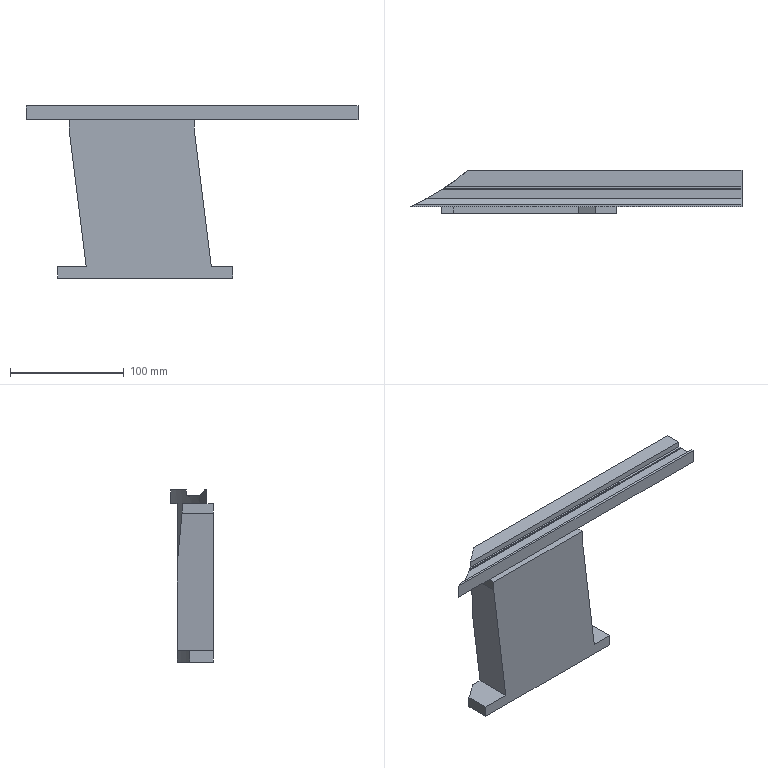Part | NX | 1 solid | 28 faces | box 291.899 x 37.727 x 151.4 mm | volume 585799 mm3 | plane 26 | cylinder 2 | commonest cylinder face diameters 412 x2
STEP:
#1=CARTESIAN_POINT('',(458.332,-185.564,-0.6));
#2=VERTEX_POINT('',#1);
#3=CARTESIAN_POINT('',(314.332,-185.564,-0.6));
#4=VERTEX_POINT('',#3);
#5=CARTESIAN_POINT('',(-273.242,-185.564,-0.6));
#6=DIRECTION('',(-1.,0.,0.));
#7=VECTOR('',#6,1000.);
#8=LINE('',#5,#7);
#9=EDGE_CURVE('',#2,#4,#8,.T.);
#10=ORIENTED_EDGE('',*,*,#9,.F.);
#11=CARTESIAN_POINT('',(458.332,-185.564,11.4));
#12=VERTEX_POINT('',#11);
#13=CARTESIAN_POINT('',(458.332,-185.564,0.));
#14=DIRECTION('',(0.,0.,1.));
#15=VECTOR('',#14,1000.);
#16=LINE('',#13,#15);
#17=EDGE_CURVE('',#2,#12,#16,.T.);
#18=ORIENTED_EDGE('',*,*,#17,.T.);
#19=CARTESIAN_POINT('',(166.433,-185.564,11.4));
#20=VERTEX_POINT('',#19);
#21=CARTESIAN_POINT('',(-273.242,-185.564,11.4));
#22=DIRECTION('',(1.,0.,0.));
#23=VECTOR('',#22,1000.);
#24=LINE('',#21,#23);
#25=EDGE_CURVE('',#20,#12,#24,.T.);
#26=ORIENTED_EDGE('',*,*,#25,.F.);
#27=CARTESIAN_POINT('',(166.433,-185.564,-0.6));
#28=VERTEX_POINT('',#27);
#29=CARTESIAN_POINT('',(166.433,-185.564,-155.14));
#30=DIRECTION('',(0.,0.,1.));
#31=VECTOR('',#30,1000.);
#32=LINE('',#29,#31);
#33=EDGE_CURVE('',#28,#20,#32,.T.);
#34=ORIENTED_EDGE('',*,*,#33,.F.);
#35=CARTESIAN_POINT('',(204.332,-185.564,-0.6));
#36=VERTEX_POINT('',#35);
#37=CARTESIAN_POINT('',(-273.242,-185.564,-0.6));
#38=DIRECTION('',(-1.,0.,0.));
#39=VECTOR('',#38,1000.);
#40=LINE('',#37,#39);
#41=EDGE_CURVE('',#36,#28,#40,.T.);
#42=ORIENTED_EDGE('',*,*,#41,.F.);
#43=CARTESIAN_POINT('',(-273.242,-185.564,-0.6));
#44=DIRECTION('',(-1.,0.,0.));
#45=VECTOR('',#44,1000.);
#46=LINE('',#43,#45);
#47=EDGE_CURVE('',#4,#36,#46,.T.);
#48=ORIENTED_EDGE('',*,*,#47,.F.);
#49=EDGE_LOOP('',(#10,#18,#26,#34,#42,#48));
#50=FACE_BOUND('',#49,.T.);
#51=CARTESIAN_POINT('',(384.332,-185.564,0.));
#52=DIRECTION('',(0.,-1.,0.));
#53=DIRECTION('',(0.,0.,-1.));
#54=AXIS2_PLACEMENT_3D('',#51,#52,#53);
#55=PLANE('',#54);
#56=ADVANCED_FACE('',(#50),#55,.T.);
#57=CARTESIAN_POINT('',(458.332,-153.564,-0.6));
#58=VERTEX_POINT('',#57);
#59=CARTESIAN_POINT('',(458.332,-346.647,-0.6));
#60=DIRECTION('',(0.,1.,0.));
#61=VECTOR('',#60,1000.);
#62=LINE('',#59,#61);
#63=EDGE_CURVE('',#2,#58,#62,.T.);
#64=ORIENTED_EDGE('',*,*,#63,.T.);
#65=CARTESIAN_POINT('',(458.332,-153.564,11.4));
#66=VERTEX_POINT('',#65);
#67=CARTESIAN_POINT('',(458.332,-153.564,0.));
#68=DIRECTION('',(0.,0.,-1.));
#69=VECTOR('',#68,1000.);
#70=LINE('',#67,#69);
#71=EDGE_CURVE('',#66,#58,#70,.T.);
#72=ORIENTED_EDGE('',*,*,#71,.F.);
#73=CARTESIAN_POINT('',(458.332,-167.364,11.4));
#74=VERTEX_POINT('',#73);
#75=CARTESIAN_POINT('',(458.332,-346.647,11.4));
#76=DIRECTION('',(0.,1.,0.));
#77=VECTOR('',#76,1000.);
#78=LINE('',#75,#77);
#79=EDGE_CURVE('',#74,#66,#78,.T.);
#80=ORIENTED_EDGE('',*,*,#79,.F.);
#81=CARTESIAN_POINT('',(458.332,-167.364,6.3));
#82=VERTEX_POINT('',#81);
#83=CARTESIAN_POINT('',(458.332,-167.364,0.));
#84=DIRECTION('',(0.,0.,-1.));
#85=VECTOR('',#84,1000.);
#86=LINE('',#83,#85);
#87=EDGE_CURVE('',#74,#82,#86,.T.);
#88=ORIENTED_EDGE('',*,*,#87,.T.);
#89=CARTESIAN_POINT('',(458.332,-169.164,6.3));
#90=VERTEX_POINT('',#89);
#91=CARTESIAN_POINT('',(458.332,-346.647,6.3));
#92=DIRECTION('',(0.,-1.,0.));
#93=VECTOR('',#92,1000.);
#94=LINE('',#91,#93);
#95=EDGE_CURVE('',#82,#90,#94,.T.);
#96=ORIENTED_EDGE('',*,*,#95,.T.);
#97=CARTESIAN_POINT('',(458.332,-169.164,5.5));
#98=VERTEX_POINT('',#97);
#99=CARTESIAN_POINT('',(458.332,-169.164,0.));
#100=DIRECTION('',(0.,0.,-1.));
#101=VECTOR('',#100,1000.);
#102=LINE('',#99,#101);
#103=EDGE_CURVE('',#90,#98,#102,.T.);
#104=ORIENTED_EDGE('',*,*,#103,.T.);
#105=CARTESIAN_POINT('',(458.332,-170.364,5.5));
#106=VERTEX_POINT('',#105);
#107=CARTESIAN_POINT('',(458.332,-346.647,5.5));
#108=DIRECTION('',(0.,-1.,0.));
#109=VECTOR('',#108,1000.);
#110=LINE('',#107,#109);
#111=EDGE_CURVE('',#98,#106,#110,.T.);
#112=ORIENTED_EDGE('',*,*,#111,.T.);
#113=CARTESIAN_POINT('',(458.332,-170.364,6.3));
#114=VERTEX_POINT('',#113);
#115=CARTESIAN_POINT('',(458.332,-170.364,0.));
#116=DIRECTION('',(0.,0.,1.));
#117=VECTOR('',#116,1000.);
#118=LINE('',#115,#117);
#119=EDGE_CURVE('',#106,#114,#118,.T.);
#120=ORIENTED_EDGE('',*,*,#119,.T.);
#121=CARTESIAN_POINT('',(458.332,-178.464,6.3));
#122=VERTEX_POINT('',#121);
#123=CARTESIAN_POINT('',(458.332,-346.647,6.3));
#124=DIRECTION('',(0.,-1.,0.));
#125=VECTOR('',#124,1000.);
#126=LINE('',#123,#125);
#127=EDGE_CURVE('',#114,#122,#126,.T.);
#128=ORIENTED_EDGE('',*,*,#127,.T.);
#129=CARTESIAN_POINT('',(458.332,-183.564,11.4));
#130=VERTEX_POINT('',#129);
#131=CARTESIAN_POINT('',(458.332,-172.164,0.));
#132=DIRECTION('',(0.,0.7071,-0.7071));
#133=VECTOR('',#132,1000.);
#134=LINE('',#131,#133);
#135=EDGE_CURVE('',#130,#122,#134,.T.);
#136=ORIENTED_EDGE('',*,*,#135,.F.);
#137=CARTESIAN_POINT('',(458.332,-346.647,11.4));
#138=DIRECTION('',(0.,1.,0.));
#139=VECTOR('',#138,1000.);
#140=LINE('',#137,#139);
#141=EDGE_CURVE('',#12,#130,#140,.T.);
#142=ORIENTED_EDGE('',*,*,#141,.F.);
#143=ORIENTED_EDGE('',*,*,#17,.F.);
#144=EDGE_LOOP('',(#64,#72,#80,#88,#96,#104,#112,#120,#128,#136,#142,#143));
#145=FACE_BOUND('',#144,.T.);
#146=CARTESIAN_POINT('',(458.332,-167.291,0.));
#147=DIRECTION('',(1.,0.,0.));
#148=DIRECTION('',(0.,1.,0.));
#149=AXIS2_PLACEMENT_3D('',#146,#147,#148);
#150=PLANE('',#149);
#151=ADVANCED_FACE('',(#145),#150,.T.);
#152=CARTESIAN_POINT('',(180.874,-178.464,6.3));
#153=VERTEX_POINT('',#152);
#154=CARTESIAN_POINT('',(194.553,-170.364,6.3));
#155=VERTEX_POINT('',#154);
#156=CARTESIAN_POINT('',(82.832,2.709,6.3));
#157=DIRECTION('',(0.,0.,1.));
#158=DIRECTION('',(1.,0.,0.));
#159=AXIS2_PLACEMENT_3D('',#156,#157,#158);
#160=CIRCLE('',#159,206.);
#161=EDGE_CURVE('',#153,#155,#160,.T.);
#162=ORIENTED_EDGE('',*,*,#161,.F.);
#163=CARTESIAN_POINT('',(-273.242,-178.464,6.3));
#164=DIRECTION('',(1.,0.,0.));
#165=VECTOR('',#164,1000.);
#166=LINE('',#163,#165);
#167=EDGE_CURVE('',#153,#122,#166,.T.);
#168=ORIENTED_EDGE('',*,*,#167,.T.);
#169=ORIENTED_EDGE('',*,*,#127,.F.);
#170=CARTESIAN_POINT('',(-273.242,-170.364,6.3));
#171=DIRECTION('',(-1.,0.,0.));
#172=VECTOR('',#171,1000.);
#173=LINE('',#170,#172);
#174=EDGE_CURVE('',#114,#155,#173,.T.);
#175=ORIENTED_EDGE('',*,*,#174,.T.);
#176=EDGE_LOOP('',(#162,#168,#169,#175));
#177=FACE_BOUND('',#176,.T.);
#178=CARTESIAN_POINT('',(99.482,-167.364,6.3));
#179=DIRECTION('',(0.,0.,-1.));
#180=DIRECTION('',(0.,-1.,0.));
#181=AXIS2_PLACEMENT_3D('',#178,#179,#180);
#182=PLANE('',#181);
#183=ADVANCED_FACE('',(#177),#182,.F.);
#184=CARTESIAN_POINT('',(204.332,-163.645,-9.));
#185=VERTEX_POINT('',#184);
#186=CARTESIAN_POINT('',(204.332,-163.645,-0.6));
#187=VERTEX_POINT('',#186);
#188=CARTESIAN_POINT('',(204.332,-163.645,-155.14));
#189=DIRECTION('',(0.,0.,1.));
#190=VECTOR('',#189,1000.);
#191=LINE('',#188,#190);
#192=EDGE_CURVE('',#185,#187,#191,.T.);
#193=ORIENTED_EDGE('',*,*,#192,.F.);
#194=CARTESIAN_POINT('',(204.332,-191.291,-9.));
#195=VERTEX_POINT('',#194);
#196=CARTESIAN_POINT('',(204.332,-175.291,-9.));
#197=DIRECTION('',(0.,-1.,0.));
#198=VECTOR('',#197,1000.);
#199=LINE('',#196,#198);
#200=EDGE_CURVE('',#185,#195,#199,.T.);
#201=ORIENTED_EDGE('',*,*,#200,.T.);
#202=CARTESIAN_POINT('',(204.332,-191.291,-0.6));
#203=VERTEX_POINT('',#202);
#204=CARTESIAN_POINT('',(204.332,-191.291,0.));
#205=DIRECTION('',(0.,0.,1.));
#206=VECTOR('',#205,1000.);
#207=LINE('',#204,#206);
#208=EDGE_CURVE('',#195,#203,#207,.T.);
#209=ORIENTED_EDGE('',*,*,#208,.T.);
#210=CARTESIAN_POINT('',(204.332,-346.647,-0.6));
#211=DIRECTION('',(0.,1.,0.));
#212=VECTOR('',#211,1000.);
#213=LINE('',#210,#212);
#214=EDGE_CURVE('',#203,#36,#213,.T.);
#215=ORIENTED_EDGE('',*,*,#214,.T.);
#216=CARTESIAN_POINT('',(204.332,-346.647,-0.6));
#217=DIRECTION('',(0.,1.,0.));
#218=VECTOR('',#217,1000.);
#219=LINE('',#216,#218);
#220=EDGE_CURVE('',#36,#187,#219,.T.);
#221=ORIENTED_EDGE('',*,*,#220,.T.);
#222=EDGE_LOOP('',(#193,#201,#209,#215,#221));
#223=FACE_BOUND('',#222,.T.);
#224=CARTESIAN_POINT('',(204.332,-175.291,-9.));
#225=DIRECTION('',(-1.,0.,0.));
#226=DIRECTION('',(0.,0.,1.));
#227=AXIS2_PLACEMENT_3D('',#224,#225,#226);
#228=PLANE('',#227);
#229=ADVANCED_FACE('',(#223),#228,.T.);
#230=CARTESIAN_POINT('',(314.332,-191.291,-0.6));
#231=VERTEX_POINT('',#230);
#232=CARTESIAN_POINT('',(314.332,-346.647,-0.6));
#233=DIRECTION('',(0.,-1.,0.));
#234=VECTOR('',#233,1000.);
#235=LINE('',#232,#234);
#236=EDGE_CURVE('',#4,#231,#235,.T.);
#237=ORIENTED_EDGE('',*,*,#236,.T.);
#238=CARTESIAN_POINT('',(314.332,-191.291,-9.));
#239=VERTEX_POINT('',#238);
#240=CARTESIAN_POINT('',(314.332,-191.291,0.));
#241=DIRECTION('',(0.,0.,-1.));
#242=VECTOR('',#241,1000.);
#243=LINE('',#240,#242);
#244=EDGE_CURVE('',#231,#239,#243,.T.);
#245=ORIENTED_EDGE('',*,*,#244,.T.);
#246=CARTESIAN_POINT('',(314.332,-159.291,-9.));
#247=VERTEX_POINT('',#246);
#248=CARTESIAN_POINT('',(314.332,-175.291,-9.));
#249=DIRECTION('',(0.,-1.,0.));
#250=VECTOR('',#249,1000.);
#251=LINE('',#248,#250);
#252=EDGE_CURVE('',#247,#239,#251,.T.);
#253=ORIENTED_EDGE('',*,*,#252,.F.);
#254=CARTESIAN_POINT('',(314.332,-159.291,-0.6));
#255=VERTEX_POINT('',#254);
#256=CARTESIAN_POINT('',(314.332,-159.291,0.));
#257=DIRECTION('',(0.,0.,-1.));
#258=VECTOR('',#257,1000.);
#259=LINE('',#256,#258);
#260=EDGE_CURVE('',#255,#247,#259,.T.);
#261=ORIENTED_EDGE('',*,*,#260,.F.);
#262=CARTESIAN_POINT('',(314.332,-346.647,-0.6));
#263=DIRECTION('',(0.,-1.,0.));
#264=VECTOR('',#263,1000.);
#265=LINE('',#262,#264);
#266=EDGE_CURVE('',#255,#4,#265,.T.);
#267=ORIENTED_EDGE('',*,*,#266,.T.);
#268=EDGE_LOOP('',(#237,#245,#253,#261,#267));
#269=FACE_BOUND('',#268,.T.);
#270=CARTESIAN_POINT('',(314.332,-175.291,0.));
#271=DIRECTION('',(1.,0.,0.));
#272=DIRECTION('',(0.,1.,0.));
#273=AXIS2_PLACEMENT_3D('',#270,#271,#272);
#274=PLANE('',#273);
#275=ADVANCED_FACE('',(#269),#274,.T.);
#276=ORIENTED_EDGE('',*,*,#244,.F.);
#277=CARTESIAN_POINT('',(-273.242,-191.291,-0.6));
#278=DIRECTION('',(-1.,0.,0.));
#279=VECTOR('',#278,1000.);
#280=LINE('',#277,#279);
#281=EDGE_CURVE('',#231,#203,#280,.T.);
#282=ORIENTED_EDGE('',*,*,#281,.T.);
#283=ORIENTED_EDGE('',*,*,#208,.F.);
#284=CARTESIAN_POINT('',(219.332,-191.291,-130.));
#285=VERTEX_POINT('',#284);
#286=CARTESIAN_POINT('',(203.216,-191.291,0.));
#287=DIRECTION('',(-0.123,0.,0.9924));
#288=VECTOR('',#287,1000.);
#289=LINE('',#286,#288);
#290=EDGE_CURVE('',#285,#195,#289,.T.);
#291=ORIENTED_EDGE('',*,*,#290,.F.);
#292=CARTESIAN_POINT('',(194.332,-191.291,-130.));
#293=VERTEX_POINT('',#292);
#294=CARTESIAN_POINT('',(-273.242,-191.291,-130.));
#295=DIRECTION('',(1.,0.,0.));
#296=VECTOR('',#295,1000.);
#297=LINE('',#294,#296);
#298=EDGE_CURVE('',#293,#285,#297,.T.);
#299=ORIENTED_EDGE('',*,*,#298,.F.);
#300=CARTESIAN_POINT('',(194.332,-191.291,-140.));
#301=VERTEX_POINT('',#300);
#302=CARTESIAN_POINT('',(194.332,-191.291,0.));
#303=DIRECTION('',(0.,0.,1.));
#304=VECTOR('',#303,1000.);
#305=LINE('',#302,#304);
#306=EDGE_CURVE('',#301,#293,#305,.T.);
#307=ORIENTED_EDGE('',*,*,#306,.F.);
#308=CARTESIAN_POINT('',(348.332,-191.291,-140.));
#309=VERTEX_POINT('',#308);
#310=CARTESIAN_POINT('',(-273.242,-191.291,-140.));
#311=DIRECTION('',(-1.,0.,0.));
#312=VECTOR('',#311,1000.);
#313=LINE('',#310,#312);
#314=EDGE_CURVE('',#309,#301,#313,.T.);
#315=ORIENTED_EDGE('',*,*,#314,.F.);
#316=CARTESIAN_POINT('',(348.332,-191.291,-130.));
#317=VERTEX_POINT('',#316);
#318=CARTESIAN_POINT('',(348.332,-191.291,0.));
#319=DIRECTION('',(0.,0.,-1.));
#320=VECTOR('',#319,1000.);
#321=LINE('',#318,#320);
#322=EDGE_CURVE('',#317,#309,#321,.T.);
#323=ORIENTED_EDGE('',*,*,#322,.F.);
#324=CARTESIAN_POINT('',(329.332,-191.291,-130.));
#325=VERTEX_POINT('',#324);
#326=CARTESIAN_POINT('',(-273.242,-191.291,-130.));
#327=DIRECTION('',(1.,0.,0.));
#328=VECTOR('',#327,1000.);
#329=LINE('',#326,#328);
#330=EDGE_CURVE('',#325,#317,#329,.T.);
#331=ORIENTED_EDGE('',*,*,#330,.F.);
#332=CARTESIAN_POINT('',(313.216,-191.291,0.));
#333=DIRECTION('',(0.123,0.,-0.9924));
#334=VECTOR('',#333,1000.);
#335=LINE('',#332,#334);
#336=EDGE_CURVE('',#239,#325,#335,.T.);
#337=ORIENTED_EDGE('',*,*,#336,.F.);
#338=EDGE_LOOP('',(#276,#282,#283,#291,#299,#307,#315,#323,#331,#337));
#339=FACE_BOUND('',#338,.T.);
#340=CARTESIAN_POINT('',(377.274,-191.291,2.035));
#341=DIRECTION('',(0.,-1.,0.));
#342=DIRECTION('',(0.,0.,-1.));
#343=AXIS2_PLACEMENT_3D('',#340,#341,#342);
#344=PLANE('',#343);
#345=ADVANCED_FACE('',(#339),#344,.T.);
#346=CARTESIAN_POINT('',(348.332,-159.291,-140.));
#347=VERTEX_POINT('',#346);
#348=CARTESIAN_POINT('',(348.332,-346.647,-140.));
#349=DIRECTION('',(0.,-1.,0.));
#350=VECTOR('',#349,1000.);
#351=LINE('',#348,#350);
#352=EDGE_CURVE('',#347,#309,#351,.T.);
#353=ORIENTED_EDGE('',*,*,#352,.F.);
#354=CARTESIAN_POINT('',(348.332,-159.291,-130.));
#355=VERTEX_POINT('',#354);
#356=CARTESIAN_POINT('',(348.332,-159.291,0.));
#357=DIRECTION('',(0.,0.,-1.));
#358=VECTOR('',#357,1000.);
#359=LINE('',#356,#358);
#360=EDGE_CURVE('',#355,#347,#359,.T.);
#361=ORIENTED_EDGE('',*,*,#360,.F.);
#362=CARTESIAN_POINT('',(348.332,-346.647,-130.));
#363=DIRECTION('',(0.,-1.,0.));
#364=VECTOR('',#363,1000.);
#365=LINE('',#362,#364);
#366=EDGE_CURVE('',#355,#317,#365,.T.);
#367=ORIENTED_EDGE('',*,*,#366,.T.);
#368=ORIENTED_EDGE('',*,*,#322,.T.);
#369=EDGE_LOOP('',(#353,#361,#367,#368));
#370=FACE_BOUND('',#369,.T.);
#371=CARTESIAN_POINT('',(348.332,-175.291,-140.));
#372=DIRECTION('',(1.,0.,0.));
#373=DIRECTION('',(0.,1.,0.));
#374=AXIS2_PLACEMENT_3D('',#371,#372,#373);
#375=PLANE('',#374);
#376=ADVANCED_FACE('',(#370),#375,.T.);
#377=CARTESIAN_POINT('',(194.332,-170.507,-130.));
#378=VERTEX_POINT('',#377);
#379=CARTESIAN_POINT('',(210.08,-159.291,-130.));
#380=VERTEX_POINT('',#379);
#381=CARTESIAN_POINT('',(82.832,2.709,-130.));
#382=DIRECTION('',(0.,0.,1.));
#383=DIRECTION('',(1.,0.,0.));
#384=AXIS2_PLACEMENT_3D('',#381,#382,#383);
#385=CIRCLE('',#384,206.);
#386=EDGE_CURVE('',#378,#380,#385,.T.);
#387=ORIENTED_EDGE('',*,*,#386,.F.);
#388=CARTESIAN_POINT('',(194.332,-175.291,-130.));
#389=DIRECTION('',(0.,1.,0.));
#390=VECTOR('',#389,1000.);
#391=LINE('',#388,#390);
#392=EDGE_CURVE('',#293,#378,#391,.T.);
#393=ORIENTED_EDGE('',*,*,#392,.F.);
#394=ORIENTED_EDGE('',*,*,#298,.T.);
#395=CARTESIAN_POINT('',(219.332,-159.291,-130.));
#396=VERTEX_POINT('',#395);
#397=CARTESIAN_POINT('',(219.332,-346.647,-130.));
#398=DIRECTION('',(0.,1.,0.));
#399=VECTOR('',#398,1000.);
#400=LINE('',#397,#399);
#401=EDGE_CURVE('',#285,#396,#400,.T.);
#402=ORIENTED_EDGE('',*,*,#401,.T.);
#403=CARTESIAN_POINT('',(-273.242,-159.291,-130.));
#404=DIRECTION('',(1.,0.,0.));
#405=VECTOR('',#404,1000.);
#406=LINE('',#403,#405);
#407=EDGE_CURVE('',#380,#396,#406,.T.);
#408=ORIENTED_EDGE('',*,*,#407,.F.);
#409=EDGE_LOOP('',(#387,#393,#394,#402,#408));
#410=FACE_BOUND('',#409,.T.);
#411=CARTESIAN_POINT('',(194.332,-175.291,-130.));
#412=DIRECTION('',(0.,0.,1.));
#413=DIRECTION('',(1.,0.,0.));
#414=AXIS2_PLACEMENT_3D('',#411,#412,#413);
#415=PLANE('',#414);
#416=ADVANCED_FACE('',(#410),#415,.T.);
#417=CARTESIAN_POINT('',(329.332,-159.291,-130.));
#418=VERTEX_POINT('',#417);
#419=CARTESIAN_POINT('',(329.332,-346.647,-130.));
#420=DIRECTION('',(0.,-1.,0.));
#421=VECTOR('',#420,1000.);
#422=LINE('',#419,#421);
#423=EDGE_CURVE('',#418,#325,#422,.T.);
#424=ORIENTED_EDGE('',*,*,#423,.F.);
#425=CARTESIAN_POINT('',(313.216,-159.291,0.));
#426=DIRECTION('',(0.123,0.,-0.9924));
#427=VECTOR('',#426,1000.);
#428=LINE('',#425,#427);
#429=EDGE_CURVE('',#247,#418,#428,.T.);
#430=ORIENTED_EDGE('',*,*,#429,.F.);
#431=ORIENTED_EDGE('',*,*,#252,.T.);
#432=ORIENTED_EDGE('',*,*,#336,.T.);
#433=EDGE_LOOP('',(#424,#430,#431,#432));
#434=FACE_BOUND('',#433,.T.);
#435=CARTESIAN_POINT('',(329.332,-175.291,-130.));
#436=DIRECTION('',(0.9924,0.,0.123));
#437=DIRECTION('',(0.,-1.,0.));
#438=AXIS2_PLACEMENT_3D('',#435,#436,#437);
#439=PLANE('',#438);
#440=ADVANCED_FACE('',(#434),#439,.T.);
#441=ORIENTED_EDGE('',*,*,#47,.T.);
#442=ORIENTED_EDGE('',*,*,#214,.F.);
#443=ORIENTED_EDGE('',*,*,#281,.F.);
#444=ORIENTED_EDGE('',*,*,#236,.F.);
#445=EDGE_LOOP('',(#441,#442,#443,#444));
#446=FACE_BOUND('',#445,.T.);
#447=CARTESIAN_POINT('',(204.332,-175.291,-0.6));
#448=DIRECTION('',(0.,0.,1.));
#449=DIRECTION('',(1.,0.,0.));
#450=AXIS2_PLACEMENT_3D('',#447,#448,#449);
#451=PLANE('',#450);
#452=ADVANCED_FACE('',(#446),#451,.T.);
#453=CARTESIAN_POINT('',(210.08,-159.291,-55.366));
#454=VERTEX_POINT('',#453);
#455=CARTESIAN_POINT('',(210.08,-159.291,-0.6));
#456=VERTEX_POINT('',#455);
#457=CARTESIAN_POINT('',(210.08,-159.291,-155.14));
#458=DIRECTION('',(0.,0.,1.));
#459=VECTOR('',#458,1000.);
#460=LINE('',#457,#459);
#461=EDGE_CURVE('',#454,#456,#460,.T.);
#462=ORIENTED_EDGE('',*,*,#461,.T.);
#463=CARTESIAN_POINT('',(-273.242,-159.291,-0.6));
#464=DIRECTION('',(-1.,0.,0.));
#465=VECTOR('',#464,1000.);
#466=LINE('',#463,#465);
#467=EDGE_CURVE('',#255,#456,#466,.T.);
#468=ORIENTED_EDGE('',*,*,#467,.F.);
#469=ORIENTED_EDGE('',*,*,#260,.T.);
#470=ORIENTED_EDGE('',*,*,#429,.T.);
#471=CARTESIAN_POINT('',(-273.242,-159.291,-130.));
#472=DIRECTION('',(-1.,0.,0.));
#473=VECTOR('',#472,1000.);
#474=LINE('',#471,#473);
#475=EDGE_CURVE('',#355,#418,#474,.T.);
#476=ORIENTED_EDGE('',*,*,#475,.F.);
#477=ORIENTED_EDGE('',*,*,#360,.T.);
#478=CARTESIAN_POINT('',(210.08,-159.291,-140.));
#479=VERTEX_POINT('',#478);
#480=CARTESIAN_POINT('',(-273.242,-159.291,-140.));
#481=DIRECTION('',(-1.,0.,0.));
#482=VECTOR('',#481,1000.);
#483=LINE('',#480,#482);
#484=EDGE_CURVE('',#347,#479,#483,.T.);
#485=ORIENTED_EDGE('',*,*,#484,.T.);
#486=CARTESIAN_POINT('',(210.08,-159.291,-155.14));
#487=DIRECTION('',(0.,0.,1.));
#488=VECTOR('',#487,1000.);
#489=LINE('',#486,#488);
#490=EDGE_CURVE('',#479,#380,#489,.T.);
#491=ORIENTED_EDGE('',*,*,#490,.T.);
#492=ORIENTED_EDGE('',*,*,#407,.T.);
#493=CARTESIAN_POINT('',(203.216,-159.291,0.));
#494=DIRECTION('',(-0.123,0.,0.9924));
#495=VECTOR('',#494,1000.);
#496=LINE('',#493,#495);
#497=EDGE_CURVE('',#396,#454,#496,.T.);
#498=ORIENTED_EDGE('',*,*,#497,.T.);
#499=EDGE_LOOP('',(#462,#468,#469,#470,#476,#477,#485,#491,#492,#498));
#500=FACE_BOUND('',#499,.T.);
#501=CARTESIAN_POINT('',(377.274,-159.291,2.035));
#502=DIRECTION('',(0.,-1.,0.));
#503=DIRECTION('',(0.,0.,-1.));
#504=AXIS2_PLACEMENT_3D('',#501,#502,#503);
#505=PLANE('',#504);
#506=ADVANCED_FACE('',(#500),#505,.F.);
#507=CARTESIAN_POINT('',(217.05,-153.564,-0.6));
#508=VERTEX_POINT('',#507);
#509=CARTESIAN_POINT('',(217.05,-153.564,11.4));
#510=VERTEX_POINT('',#509);
#511=CARTESIAN_POINT('',(217.05,-153.564,-155.14));
#512=DIRECTION('',(0.,0.,1.));
#513=VECTOR('',#512,1000.);
#514=LINE('',#511,#513);
#515=EDGE_CURVE('',#508,#510,#514,.T.);
#516=ORIENTED_EDGE('',*,*,#515,.T.);
#517=CARTESIAN_POINT('',(-273.242,-153.564,11.4));
#518=DIRECTION('',(-1.,0.,0.));
#519=VECTOR('',#518,1000.);
#520=LINE('',#517,#519);
#521=EDGE_CURVE('',#66,#510,#520,.T.);
#522=ORIENTED_EDGE('',*,*,#521,.F.);
#523=ORIENTED_EDGE('',*,*,#71,.T.);
#524=CARTESIAN_POINT('',(-273.242,-153.564,-0.6));
#525=DIRECTION('',(1.,0.,0.));
#526=VECTOR('',#525,1000.);
#527=LINE('',#524,#526);
#528=EDGE_CURVE('',#508,#58,#527,.T.);
#529=ORIENTED_EDGE('',*,*,#528,.F.);
#530=EDGE_LOOP('',(#516,#522,#523,#529));
#531=FACE_BOUND('',#530,.T.);
#532=CARTESIAN_POINT('',(134.332,-153.564,0.));
#533=DIRECTION('',(0.,1.,0.));
#534=DIRECTION('',(1.,0.,0.));
#535=AXIS2_PLACEMENT_3D('',#532,#533,#534);
#536=PLANE('',#535);
#537=ADVANCED_FACE('',(#531),#536,.T.);
#538=ORIENTED_EDGE('',*,*,#200,.F.);
#539=CARTESIAN_POINT('',(210.08,-159.291,-55.366));
#540=CARTESIAN_POINT('',(208.189,-160.776,-40.116));
#541=CARTESIAN_POINT('',(206.273,-162.227,-24.659));
#542=CARTESIAN_POINT('',(204.332,-163.645,-9.));
#543=(BOUNDED_CURVE()B_SPLINE_CURVE(3,(#539,#540,#541,#542),.UNSPECIFIED.,.F.,.F.)B_SPLINE_CURVE_WITH_KNOTS((4,4),(4.047,4.082),.UNSPECIFIED.)CURVE()GEOMETRIC_REPRESENTATION_ITEM()RATIONAL_B_SPLINE_CURVE((1.,0.9999,0.9999,1.))REPRESENTATION_ITEM(''));
#544=EDGE_CURVE('',#454,#185,#543,.T.);
#545=ORIENTED_EDGE('',*,*,#544,.F.);
#546=ORIENTED_EDGE('',*,*,#497,.F.);
#547=ORIENTED_EDGE('',*,*,#401,.F.);
#548=ORIENTED_EDGE('',*,*,#290,.T.);
#549=EDGE_LOOP('',(#538,#545,#546,#547,#548));
#550=FACE_BOUND('',#549,.T.);
#551=CARTESIAN_POINT('',(204.332,-175.291,-9.));
#552=DIRECTION('',(-0.9924,0.,-0.123));
#553=DIRECTION('',(-0.123,0.,0.9924));
#554=AXIS2_PLACEMENT_3D('',#551,#552,#553);
#555=PLANE('',#554);
#556=ADVANCED_FACE('',(#550),#555,.T.);
#557=CARTESIAN_POINT('',(194.332,-170.507,-140.));
#558=VERTEX_POINT('',#557);
#559=CARTESIAN_POINT('',(194.332,-346.647,-140.));
#560=DIRECTION('',(0.,-1.,0.));
#561=VECTOR('',#560,1000.);
#562=LINE('',#559,#561);
#563=EDGE_CURVE('',#558,#301,#562,.T.);
#564=ORIENTED_EDGE('',*,*,#563,.T.);
#565=ORIENTED_EDGE('',*,*,#306,.T.);
#566=ORIENTED_EDGE('',*,*,#392,.T.);
#567=CARTESIAN_POINT('',(194.332,-170.507,-155.14));
#568=DIRECTION('',(0.,0.,1.));
#569=VECTOR('',#568,1000.);
#570=LINE('',#567,#569);
#571=EDGE_CURVE('',#558,#378,#570,.T.);
#572=ORIENTED_EDGE('',*,*,#571,.F.);
#573=EDGE_LOOP('',(#564,#565,#566,#572));
#574=FACE_BOUND('',#573,.T.);
#575=CARTESIAN_POINT('',(194.332,-175.291,-140.));
#576=DIRECTION('',(-1.,0.,0.));
#577=DIRECTION('',(0.,0.,1.));
#578=AXIS2_PLACEMENT_3D('',#575,#576,#577);
#579=PLANE('',#578);
#580=ADVANCED_FACE('',(#574),#579,.T.);
#581=ORIENTED_EDGE('',*,*,#563,.F.);
#582=CARTESIAN_POINT('',(82.832,2.709,-140.));
#583=DIRECTION('',(0.,0.,1.));
#584=DIRECTION('',(1.,0.,0.));
#585=AXIS2_PLACEMENT_3D('',#582,#583,#584);
#586=CIRCLE('',#585,206.);
#587=EDGE_CURVE('',#558,#479,#586,.T.);
#588=ORIENTED_EDGE('',*,*,#587,.T.);
#589=ORIENTED_EDGE('',*,*,#484,.F.);
#590=ORIENTED_EDGE('',*,*,#352,.T.);
#591=ORIENTED_EDGE('',*,*,#314,.T.);
#592=EDGE_LOOP('',(#581,#588,#589,#590,#591));
#593=FACE_BOUND('',#592,.T.);
#594=CARTESIAN_POINT('',(194.332,-175.291,-140.));
#595=DIRECTION('',(0.,0.,-1.));
#596=DIRECTION('',(0.,-1.,0.));
#597=AXIS2_PLACEMENT_3D('',#594,#595,#596);
#598=PLANE('',#597);
#599=ADVANCED_FACE('',(#593),#598,.T.);
#600=ORIENTED_EDGE('',*,*,#423,.T.);
#601=ORIENTED_EDGE('',*,*,#330,.T.);
#602=ORIENTED_EDGE('',*,*,#366,.F.);
#603=ORIENTED_EDGE('',*,*,#475,.T.);
#604=EDGE_LOOP('',(#600,#601,#602,#603));
#605=FACE_BOUND('',#604,.T.);
#606=CARTESIAN_POINT('',(354.332,-175.291,-130.));
#607=DIRECTION('',(0.,0.,1.));
#608=DIRECTION('',(1.,0.,0.));
#609=AXIS2_PLACEMENT_3D('',#606,#607,#608);
#610=PLANE('',#609);
#611=ADVANCED_FACE('',(#605),#610,.T.);
#612=ORIENTED_EDGE('',*,*,#167,.F.);
#613=CARTESIAN_POINT('',(170.799,-183.564,11.4));
#614=VERTEX_POINT('',#613);
#615=CARTESIAN_POINT('',(170.799,-183.564,11.4));
#616=CARTESIAN_POINT('',(174.203,-181.957,9.792));
#617=CARTESIAN_POINT('',(177.562,-180.256,8.092));
#618=CARTESIAN_POINT('',(180.874,-178.464,6.3));
#619=(BOUNDED_CURVE()B_SPLINE_CURVE(3,(#615,#616,#617,#618),.UNSPECIFIED.,.F.,.F.)B_SPLINE_CURVE_WITH_KNOTS((4,4),(0.4412,0.496),.UNSPECIFIED.)CURVE()GEOMETRIC_REPRESENTATION_ITEM()RATIONAL_B_SPLINE_CURVE((1.,0.9997,0.9997,1.))REPRESENTATION_ITEM(''));
#620=EDGE_CURVE('',#614,#153,#619,.T.);
#621=ORIENTED_EDGE('',*,*,#620,.F.);
#622=CARTESIAN_POINT('',(-273.242,-183.564,11.4));
#623=DIRECTION('',(1.,0.,0.));
#624=VECTOR('',#623,1000.);
#625=LINE('',#622,#624);
#626=EDGE_CURVE('',#614,#130,#625,.T.);
#627=ORIENTED_EDGE('',*,*,#626,.T.);
#628=ORIENTED_EDGE('',*,*,#135,.T.);
#629=EDGE_LOOP('',(#612,#621,#627,#628));
#630=FACE_BOUND('',#629,.T.);
#631=CARTESIAN_POINT('',(308.582,-181.014,8.85));
#632=DIRECTION('',(0.,0.7071,0.7071));
#633=DIRECTION('',(1.,0.,0.));
#634=AXIS2_PLACEMENT_3D('',#631,#632,#633);
#635=PLANE('',#634);
#636=ADVANCED_FACE('',(#630),#635,.T.);
#637=ORIENTED_EDGE('',*,*,#87,.F.);
#638=CARTESIAN_POINT('',(199.069,-167.364,11.4));
#639=VERTEX_POINT('',#638);
#640=CARTESIAN_POINT('',(-273.242,-167.364,11.4));
#641=DIRECTION('',(-1.,0.,0.));
#642=VECTOR('',#641,1000.);
#643=LINE('',#640,#642);
#644=EDGE_CURVE('',#74,#639,#643,.T.);
#645=ORIENTED_EDGE('',*,*,#644,.T.);
#646=CARTESIAN_POINT('',(199.069,-167.364,6.3));
#647=VERTEX_POINT('',#646);
#648=CARTESIAN_POINT('',(199.069,-167.364,-155.14));
#649=DIRECTION('',(0.,0.,1.));
#650=VECTOR('',#649,1000.);
#651=LINE('',#648,#650);
#652=EDGE_CURVE('',#647,#639,#651,.T.);
#653=ORIENTED_EDGE('',*,*,#652,.F.);
#654=CARTESIAN_POINT('',(-273.242,-167.364,6.3));
#655=DIRECTION('',(1.,0.,0.));
#656=VECTOR('',#655,1000.);
#657=LINE('',#654,#656);
#658=EDGE_CURVE('',#647,#82,#657,.T.);
#659=ORIENTED_EDGE('',*,*,#658,.T.);
#660=EDGE_LOOP('',(#637,#645,#653,#659));
#661=FACE_BOUND('',#660,.T.);
#662=CARTESIAN_POINT('',(99.482,-167.364,20.8));
#663=DIRECTION('',(0.,1.,0.));
#664=DIRECTION('',(1.,0.,0.));
#665=AXIS2_PLACEMENT_3D('',#662,#663,#664);
#666=PLANE('',#665);
#667=ADVANCED_FACE('',(#661),#666,.F.);
#668=CARTESIAN_POINT('',(194.553,-170.364,5.5));
#669=VERTEX_POINT('',#668);
#670=CARTESIAN_POINT('',(196.39,-169.164,5.5));
#671=VERTEX_POINT('',#670);
#672=CARTESIAN_POINT('',(82.832,2.709,5.5));
#673=DIRECTION('',(0.,0.,1.));
#674=DIRECTION('',(1.,0.,0.));
#675=AXIS2_PLACEMENT_3D('',#672,#673,#674);
#676=CIRCLE('',#675,206.);
#677=EDGE_CURVE('',#669,#671,#676,.T.);
#678=ORIENTED_EDGE('',*,*,#677,.F.);
#679=CARTESIAN_POINT('',(-273.242,-170.364,5.5));
#680=DIRECTION('',(1.,0.,0.));
#681=VECTOR('',#680,1000.);
#682=LINE('',#679,#681);
#683=EDGE_CURVE('',#669,#106,#682,.T.);
#684=ORIENTED_EDGE('',*,*,#683,.T.);
#685=ORIENTED_EDGE('',*,*,#111,.F.);
#686=CARTESIAN_POINT('',(-273.242,-169.164,5.5));
#687=DIRECTION('',(1.,0.,0.));
#688=VECTOR('',#687,1000.);
#689=LINE('',#686,#688);
#690=EDGE_CURVE('',#671,#98,#689,.T.);
#691=ORIENTED_EDGE('',*,*,#690,.F.);
#692=EDGE_LOOP('',(#678,#684,#685,#691));
#693=FACE_BOUND('',#692,.T.);
#694=CARTESIAN_POINT('',(99.482,-169.164,5.5));
#695=DIRECTION('',(0.,0.,-1.));
#696=DIRECTION('',(0.,-1.,0.));
#697=AXIS2_PLACEMENT_3D('',#694,#695,#696);
#698=PLANE('',#697);
#699=ADVANCED_FACE('',(#693),#698,.F.);
#700=CARTESIAN_POINT('',(196.39,-169.164,6.3));
#701=VERTEX_POINT('',#700);
#702=CARTESIAN_POINT('',(-273.242,-169.164,6.3));
#703=DIRECTION('',(1.,0.,0.));
#704=VECTOR('',#703,1000.);
#705=LINE('',#702,#704);
#706=EDGE_CURVE('',#701,#90,#705,.T.);
#707=ORIENTED_EDGE('',*,*,#706,.T.);
#708=ORIENTED_EDGE('',*,*,#95,.F.);
#709=ORIENTED_EDGE('',*,*,#658,.F.);
#710=CARTESIAN_POINT('',(82.832,2.709,6.3));
#711=DIRECTION('',(0.,0.,1.));
#712=DIRECTION('',(1.,0.,0.));
#713=AXIS2_PLACEMENT_3D('',#710,#711,#712);
#714=CIRCLE('',#713,206.);
#715=EDGE_CURVE('',#701,#647,#714,.T.);
#716=ORIENTED_EDGE('',*,*,#715,.F.);
#717=EDGE_LOOP('',(#707,#708,#709,#716));
#718=FACE_BOUND('',#717,.T.);
#719=CARTESIAN_POINT('',(99.482,-167.364,6.3));
#720=DIRECTION('',(0.,0.,-1.));
#721=DIRECTION('',(0.,-1.,0.));
#722=AXIS2_PLACEMENT_3D('',#719,#720,#721);
#723=PLANE('',#722);
#724=ADVANCED_FACE('',(#718),#723,.F.);
#725=ORIENTED_EDGE('',*,*,#119,.F.);
#726=ORIENTED_EDGE('',*,*,#683,.F.);
#727=CARTESIAN_POINT('',(194.553,-170.364,-155.14));
#728=DIRECTION('',(0.,0.,1.));
#729=VECTOR('',#728,1000.);
#730=LINE('',#727,#729);
#731=EDGE_CURVE('',#669,#155,#730,.T.);
#732=ORIENTED_EDGE('',*,*,#731,.T.);
#733=ORIENTED_EDGE('',*,*,#174,.F.);
#734=EDGE_LOOP('',(#725,#726,#732,#733));
#735=FACE_BOUND('',#734,.T.);
#736=CARTESIAN_POINT('',(99.482,-170.364,5.5));
#737=DIRECTION('',(0.,-1.,0.));
#738=DIRECTION('',(0.,0.,-1.));
#739=AXIS2_PLACEMENT_3D('',#736,#737,#738);
#740=PLANE('',#739);
#741=ADVANCED_FACE('',(#735),#740,.F.);
#742=ORIENTED_EDGE('',*,*,#103,.F.);
#743=ORIENTED_EDGE('',*,*,#706,.F.);
#744=CARTESIAN_POINT('',(196.39,-169.164,-155.14));
#745=DIRECTION('',(0.,0.,1.));
#746=VECTOR('',#745,1000.);
#747=LINE('',#744,#746);
#748=EDGE_CURVE('',#671,#701,#747,.T.);
#749=ORIENTED_EDGE('',*,*,#748,.F.);
#750=ORIENTED_EDGE('',*,*,#690,.T.);
#751=EDGE_LOOP('',(#742,#743,#749,#750));
#752=FACE_BOUND('',#751,.T.);
#753=CARTESIAN_POINT('',(99.482,-169.164,6.3));
#754=DIRECTION('',(0.,1.,0.));
#755=DIRECTION('',(1.,0.,0.));
#756=AXIS2_PLACEMENT_3D('',#753,#754,#755);
#757=PLANE('',#756);
#758=ADVANCED_FACE('',(#752),#757,.F.);
#759=ORIENTED_EDGE('',*,*,#571,.T.);
#760=ORIENTED_EDGE('',*,*,#386,.T.);
#761=ORIENTED_EDGE('',*,*,#490,.F.);
#762=ORIENTED_EDGE('',*,*,#587,.F.);
#763=EDGE_LOOP('',(#759,#760,#761,#762));
#764=FACE_BOUND('',#763,.T.);
#765=CARTESIAN_POINT('',(82.832,2.709,-155.14));
#766=DIRECTION('',(0.,0.,1.));
#767=DIRECTION('',(1.,0.,0.));
#768=AXIS2_PLACEMENT_3D('',#765,#766,#767);
#769=CYLINDRICAL_SURFACE('',#768,206.);
#770=ADVANCED_FACE('',(#764),#769,.F.);
#771=ORIENTED_EDGE('',*,*,#461,.F.);
#772=ORIENTED_EDGE('',*,*,#544,.T.);
#773=ORIENTED_EDGE('',*,*,#192,.T.);
#774=CARTESIAN_POINT('',(82.832,2.709,-0.6));
#775=DIRECTION('',(0.,0.,1.));
#776=DIRECTION('',(1.,0.,0.));
#777=AXIS2_PLACEMENT_3D('',#774,#775,#776);
#778=CIRCLE('',#777,206.);
#779=EDGE_CURVE('',#28,#187,#778,.T.);
#780=ORIENTED_EDGE('',*,*,#779,.F.);
#781=ORIENTED_EDGE('',*,*,#33,.T.);
#782=CARTESIAN_POINT('',(82.832,2.709,11.4));
#783=DIRECTION('',(0.,0.,1.));
#784=DIRECTION('',(1.,0.,0.));
#785=AXIS2_PLACEMENT_3D('',#782,#783,#784);
#786=CIRCLE('',#785,206.);
#787=EDGE_CURVE('',#20,#614,#786,.T.);
#788=ORIENTED_EDGE('',*,*,#787,.T.);
#789=ORIENTED_EDGE('',*,*,#620,.T.);
#790=ORIENTED_EDGE('',*,*,#161,.T.);
#791=ORIENTED_EDGE('',*,*,#731,.F.);
#792=ORIENTED_EDGE('',*,*,#677,.T.);
#793=ORIENTED_EDGE('',*,*,#748,.T.);
#794=ORIENTED_EDGE('',*,*,#715,.T.);
#795=ORIENTED_EDGE('',*,*,#652,.T.);
#796=CARTESIAN_POINT('',(82.832,2.709,11.4));
#797=DIRECTION('',(0.,0.,1.));
#798=DIRECTION('',(1.,0.,0.));
#799=AXIS2_PLACEMENT_3D('',#796,#797,#798);
#800=CIRCLE('',#799,206.);
#801=EDGE_CURVE('',#639,#510,#800,.T.);
#802=ORIENTED_EDGE('',*,*,#801,.T.);
#803=ORIENTED_EDGE('',*,*,#515,.F.);
#804=CARTESIAN_POINT('',(82.832,2.709,-0.6));
#805=DIRECTION('',(0.,0.,1.));
#806=DIRECTION('',(1.,0.,0.));
#807=AXIS2_PLACEMENT_3D('',#804,#805,#806);
#808=CIRCLE('',#807,206.);
#809=EDGE_CURVE('',#456,#508,#808,.T.);
#810=ORIENTED_EDGE('',*,*,#809,.F.);
#811=EDGE_LOOP('',(#771,#772,#773,#780,#781,#788,#789,#790,#791,#792,#793,#794,#795,#802,#803,#810));
#812=FACE_BOUND('',#811,.T.);
#813=CARTESIAN_POINT('',(82.832,2.709,-155.14));
#814=DIRECTION('',(0.,0.,1.));
#815=DIRECTION('',(1.,0.,0.));
#816=AXIS2_PLACEMENT_3D('',#813,#814,#815);
#817=CYLINDRICAL_SURFACE('',#816,206.);
#818=ADVANCED_FACE('',(#812),#817,.F.);
#819=ORIENTED_EDGE('',*,*,#25,.T.);
#820=ORIENTED_EDGE('',*,*,#141,.T.);
#821=ORIENTED_EDGE('',*,*,#626,.F.);
#822=ORIENTED_EDGE('',*,*,#787,.F.);
#823=EDGE_LOOP('',(#819,#820,#821,#822));
#824=FACE_BOUND('',#823,.T.);
#825=CARTESIAN_POINT('',(-273.242,-346.647,11.4));
#826=DIRECTION('',(0.,0.,1.));
#827=DIRECTION('',(1.,0.,0.));
#828=AXIS2_PLACEMENT_3D('',#825,#826,#827);
#829=PLANE('',#828);
#830=ADVANCED_FACE('',(#824),#829,.T.);
#831=ORIENTED_EDGE('',*,*,#801,.F.);
#832=ORIENTED_EDGE('',*,*,#644,.F.);
#833=ORIENTED_EDGE('',*,*,#79,.T.);
#834=ORIENTED_EDGE('',*,*,#521,.T.);
#835=EDGE_LOOP('',(#831,#832,#833,#834));
#836=FACE_BOUND('',#835,.T.);
#837=CARTESIAN_POINT('',(-273.242,-346.647,11.4));
#838=DIRECTION('',(0.,0.,1.));
#839=DIRECTION('',(1.,0.,0.));
#840=AXIS2_PLACEMENT_3D('',#837,#838,#839);
#841=PLANE('',#840);
#842=ADVANCED_FACE('',(#836),#841,.T.);
#843=ORIENTED_EDGE('',*,*,#266,.F.);
#844=ORIENTED_EDGE('',*,*,#467,.T.);
#845=ORIENTED_EDGE('',*,*,#809,.T.);
#846=ORIENTED_EDGE('',*,*,#528,.T.);
#847=ORIENTED_EDGE('',*,*,#63,.F.);
#848=ORIENTED_EDGE('',*,*,#9,.T.);
#849=EDGE_LOOP('',(#843,#844,#845,#846,#847,#848));
#850=FACE_BOUND('',#849,.T.);
#851=CARTESIAN_POINT('',(-273.242,-346.647,-0.6));
#852=DIRECTION('',(0.,0.,1.));
#853=DIRECTION('',(1.,0.,0.));
#854=AXIS2_PLACEMENT_3D('',#851,#852,#853);
#855=PLANE('',#854);
#856=ADVANCED_FACE('',(#850),#855,.F.);
#857=ORIENTED_EDGE('',*,*,#779,.T.);
#858=ORIENTED_EDGE('',*,*,#220,.F.);
#859=ORIENTED_EDGE('',*,*,#41,.T.);
#860=EDGE_LOOP('',(#857,#858,#859));
#861=FACE_BOUND('',#860,.T.);
#862=CARTESIAN_POINT('',(-273.242,-346.647,-0.6));
#863=DIRECTION('',(0.,0.,1.));
#864=DIRECTION('',(1.,0.,0.));
#865=AXIS2_PLACEMENT_3D('',#862,#863,#864);
#866=PLANE('',#865);
#867=ADVANCED_FACE('',(#861),#866,.F.);
#868=CLOSED_SHELL('',(#56,#151,#183,#229,#275,#345,#376,#416,#440,#452,#506,#537,#556,#580,#599,#611,#636,#667,#699,#724,#741,#758,#770,#818,#830,#842,#856,#867));
#869=MANIFOLD_SOLID_BREP('',#868);
#870=(LENGTH_UNIT()NAMED_UNIT(*)SI_UNIT(.MILLI.,.METRE.));
#871=UNCERTAINTY_MEASURE_WITH_UNIT(LENGTH_MEASURE(0.00001),#870,'','');
#872=(NAMED_UNIT(*)PLANE_ANGLE_UNIT()SI_UNIT($,.RADIAN.));
#873=(NAMED_UNIT(*)SI_UNIT($,.STERADIAN.)SOLID_ANGLE_UNIT());
#874=(GEOMETRIC_REPRESENTATION_CONTEXT(3)GLOBAL_UNCERTAINTY_ASSIGNED_CONTEXT((#871))GLOBAL_UNIT_ASSIGNED_CONTEXT((#870,#872,#873))REPRESENTATION_CONTEXT('',''));
#875=ADVANCED_BREP_SHAPE_REPRESENTATION('',(#869),#874);